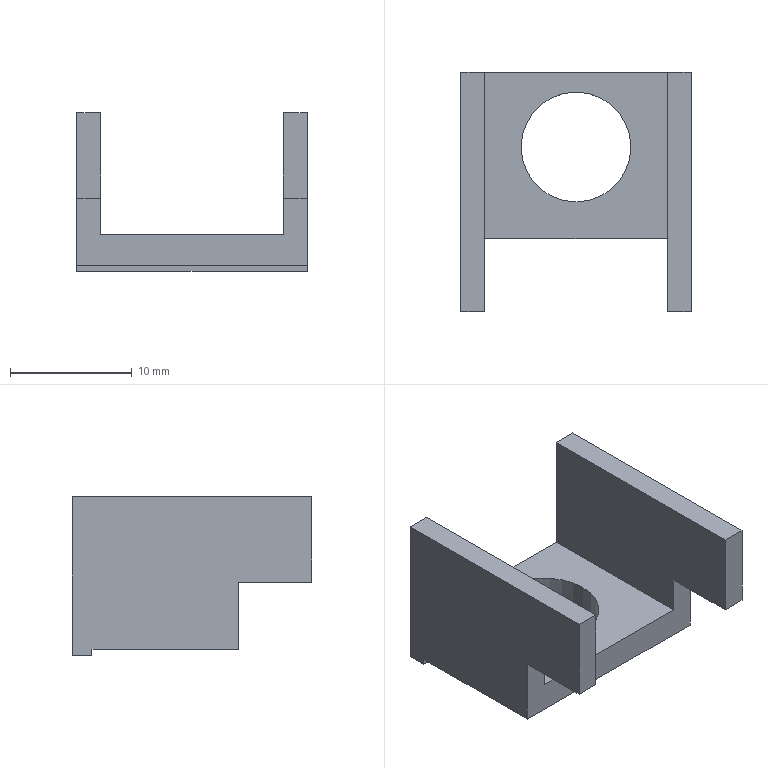Part | NX | features 18 2 | 1 solid | 69 faces | box 18.9 x 19.6 x 13 mm | volume 1192 mm3 | plane 43 | spline 24 | cylinder 2 | commonest cylinder face diameters 9 x2